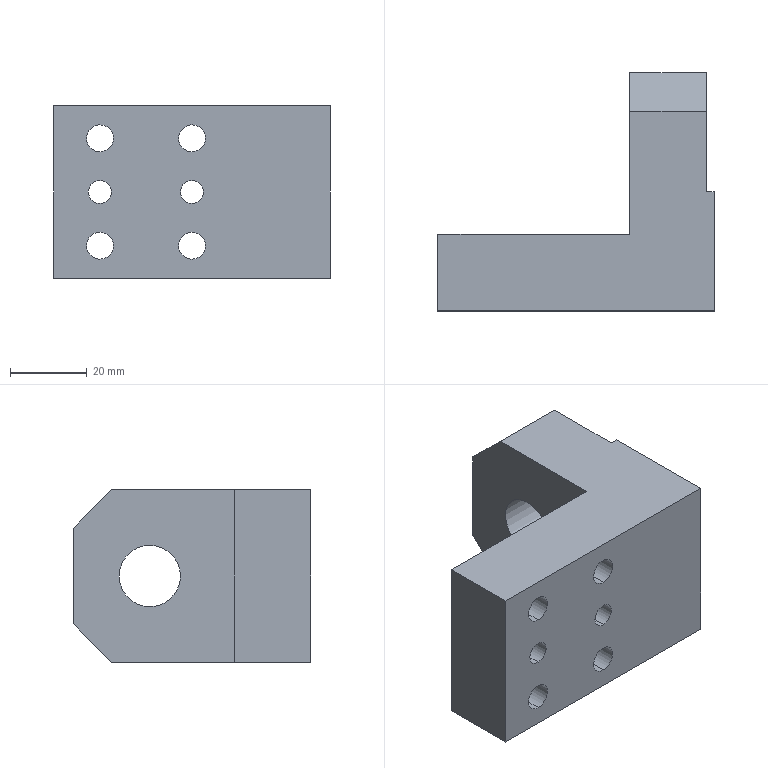Part | STEP file | Positioning_id1814_x_t | 1 solid | 26 faces | box 72 x 62 x 45 mm | volume 93359 mm3 | cylinder 14 | plane 12 | commonest cylinder face diameters 7 x8 6 x4 16 x2